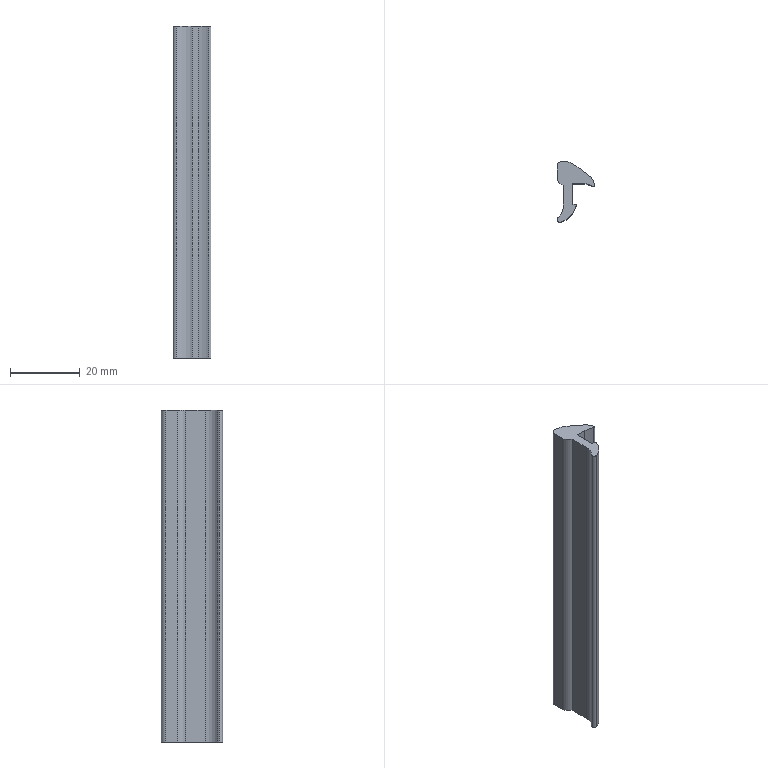Part | SolidWorks | features MoveFace 2, BaseBody 1 | 1 solid | 20 faces | box 10.8 x 17.5 x 95 mm | volume 7486 mm3 | cylinder 11 | plane 9 | commonest cylinder face diameters 1.6 x2 14 x2 0.4 x1 0.6 x1 0.8 x1 2.6 x1
STEP:
#1=CARTESIAN_POINT('',(-3.236,-11.055,115.));
#2=VERTEX_POINT('',#1);
#3=CARTESIAN_POINT('',(-4.3,-10.3,115.));
#4=VERTEX_POINT('',#3);
#5=CARTESIAN_POINT('',(-3.5,-10.3,115.));
#6=DIRECTION('',(0.,0.,-1.));
#7=DIRECTION('',(1.,0.,0.));
#8=AXIS2_PLACEMENT_3D('',#5,#6,#7);
#9=CIRCLE('',#8,0.8);
#10=EDGE_CURVE('',#2,#4,#9,.T.);
#11=ORIENTED_EDGE('',*,*,#10,.T.);
#12=CARTESIAN_POINT('',(-4.3,-10.3,20.));
#13=VERTEX_POINT('',#12);
#14=CARTESIAN_POINT('',(-4.3,-10.3,-100.));
#15=DIRECTION('',(0.,0.,-1.));
#16=VECTOR('',#15,1000.);
#17=LINE('',#14,#16);
#18=EDGE_CURVE('',#4,#13,#17,.T.);
#19=ORIENTED_EDGE('',*,*,#18,.T.);
#20=CARTESIAN_POINT('',(-3.236,-11.055,20.));
#21=VERTEX_POINT('',#20);
#22=CARTESIAN_POINT('',(-3.5,-10.3,20.));
#23=DIRECTION('',(0.,0.,1.));
#24=DIRECTION('',(1.,0.,0.));
#25=AXIS2_PLACEMENT_3D('',#22,#23,#24);
#26=CIRCLE('',#25,0.8);
#27=EDGE_CURVE('',#13,#21,#26,.T.);
#28=ORIENTED_EDGE('',*,*,#27,.T.);
#29=CARTESIAN_POINT('',(-3.236,-11.055,-100.));
#30=DIRECTION('',(0.,0.,-1.));
#31=VECTOR('',#30,1000.);
#32=LINE('',#29,#31);
#33=EDGE_CURVE('',#2,#21,#32,.T.);
#34=ORIENTED_EDGE('',*,*,#33,.F.);
#35=EDGE_LOOP('',(#11,#19,#28,#34));
#36=FACE_OUTER_BOUND('',#35,.T.);
#37=CARTESIAN_POINT('',(-3.5,-10.3,-100.));
#38=DIRECTION('',(0.,0.,-1.));
#39=DIRECTION('',(-1.,0.,0.));
#40=AXIS2_PLACEMENT_3D('',#37,#38,#39);
#41=CYLINDRICAL_SURFACE('',#40,0.8);
#42=ADVANCED_FACE('',(#36),#41,.T.);
#43=CARTESIAN_POINT('',(1.184,-6.397,20.));
#44=VERTEX_POINT('',#43);
#45=CARTESIAN_POINT('',(-5.702,-4.29,20.));
#46=DIRECTION('',(0.,0.,1.));
#47=DIRECTION('',(1.,0.,0.));
#48=AXIS2_PLACEMENT_3D('',#45,#46,#47);
#49=CIRCLE('',#48,7.201);
#50=EDGE_CURVE('',#21,#44,#49,.T.);
#51=ORIENTED_EDGE('',*,*,#50,.T.);
#52=CARTESIAN_POINT('',(1.184,-6.397,115.));
#53=VERTEX_POINT('',#52);
#54=CARTESIAN_POINT('',(1.184,-6.397,-100.));
#55=DIRECTION('',(0.,0.,1.));
#56=VECTOR('',#55,1000.);
#57=LINE('',#54,#56);
#58=EDGE_CURVE('',#44,#53,#57,.T.);
#59=ORIENTED_EDGE('',*,*,#58,.T.);
#60=CARTESIAN_POINT('',(-5.702,-4.29,115.));
#61=DIRECTION('',(0.,0.,-1.));
#62=DIRECTION('',(1.,0.,0.));
#63=AXIS2_PLACEMENT_3D('',#60,#61,#62);
#64=CIRCLE('',#63,7.201);
#65=EDGE_CURVE('',#53,#2,#64,.T.);
#66=ORIENTED_EDGE('',*,*,#65,.T.);
#67=ORIENTED_EDGE('',*,*,#33,.T.);
#68=EDGE_LOOP('',(#51,#59,#66,#67));
#69=FACE_OUTER_BOUND('',#68,.T.);
#70=CARTESIAN_POINT('',(-5.702,-4.29,-100.));
#71=DIRECTION('',(0.,0.,-1.));
#72=DIRECTION('',(-1.,0.,0.));
#73=AXIS2_PLACEMENT_3D('',#70,#71,#72);
#74=CYLINDRICAL_SURFACE('',#73,7.201);
#75=ADVANCED_FACE('',(#69),#74,.T.);
#76=CARTESIAN_POINT('',(0.9,-6.,20.));
#77=VERTEX_POINT('',#76);
#78=CARTESIAN_POINT('',(0.9,-6.3,20.));
#79=DIRECTION('',(0.,0.,1.));
#80=DIRECTION('',(1.,0.,0.));
#81=AXIS2_PLACEMENT_3D('',#78,#79,#80);
#82=CIRCLE('',#81,0.3);
#83=EDGE_CURVE('',#44,#77,#82,.T.);
#84=ORIENTED_EDGE('',*,*,#83,.T.);
#85=CARTESIAN_POINT('',(0.9,-6.,115.));
#86=VERTEX_POINT('',#85);
#87=CARTESIAN_POINT('',(0.9,-6.,-100.));
#88=DIRECTION('',(0.,0.,1.));
#89=VECTOR('',#88,1000.);
#90=LINE('',#87,#89);
#91=EDGE_CURVE('',#77,#86,#90,.T.);
#92=ORIENTED_EDGE('',*,*,#91,.T.);
#93=CARTESIAN_POINT('',(0.9,-6.3,115.));
#94=DIRECTION('',(0.,0.,-1.));
#95=DIRECTION('',(1.,0.,0.));
#96=AXIS2_PLACEMENT_3D('',#93,#94,#95);
#97=CIRCLE('',#96,0.3);
#98=EDGE_CURVE('',#86,#53,#97,.T.);
#99=ORIENTED_EDGE('',*,*,#98,.T.);
#100=ORIENTED_EDGE('',*,*,#58,.F.);
#101=EDGE_LOOP('',(#84,#92,#99,#100));
#102=FACE_OUTER_BOUND('',#101,.T.);
#103=CARTESIAN_POINT('',(0.9,-6.3,-100.));
#104=DIRECTION('',(0.,0.,-1.));
#105=DIRECTION('',(-1.,0.,0.));
#106=AXIS2_PLACEMENT_3D('',#103,#104,#105);
#107=CYLINDRICAL_SURFACE('',#106,0.3);
#108=ADVANCED_FACE('',(#102),#107,.T.);
#109=CARTESIAN_POINT('',(-2.5,-0.5,20.));
#110=VERTEX_POINT('',#109);
#111=CARTESIAN_POINT('',(-2.5,-6.153,20.));
#112=VERTEX_POINT('',#111);
#113=CARTESIAN_POINT('',(-2.5,-6.397,20.));
#114=DIRECTION('',(0.,-1.,0.));
#115=VECTOR('',#114,1000.);
#116=LINE('',#113,#115);
#117=EDGE_CURVE('',#110,#112,#116,.T.);
#118=ORIENTED_EDGE('',*,*,#117,.F.);
#119=CARTESIAN_POINT('',(-4.2,1.695,20.));
#120=VERTEX_POINT('',#119);
#121=CARTESIAN_POINT('',(-1.701,1.875,20.));
#122=DIRECTION('',(0.,0.,1.));
#123=DIRECTION('',(1.,0.,0.));
#124=AXIS2_PLACEMENT_3D('',#121,#122,#123);
#125=CIRCLE('',#124,2.506);
#126=EDGE_CURVE('',#120,#110,#125,.T.);
#127=ORIENTED_EDGE('',*,*,#126,.F.);
#128=CARTESIAN_POINT('',(-4.2,5.1,20.));
#129=VERTEX_POINT('',#128);
#130=CARTESIAN_POINT('',(-4.2,-6.397,20.));
#131=DIRECTION('',(0.,-1.,0.));
#132=VECTOR('',#131,1000.);
#133=LINE('',#130,#132);
#134=EDGE_CURVE('',#129,#120,#133,.T.);
#135=ORIENTED_EDGE('',*,*,#134,.F.);
#136=CARTESIAN_POINT('',(-2.892,6.4,20.));
#137=VERTEX_POINT('',#136);
#138=CARTESIAN_POINT('',(-2.9,5.1,20.));
#139=DIRECTION('',(0.,0.,1.));
#140=DIRECTION('',(1.,0.,0.));
#141=AXIS2_PLACEMENT_3D('',#138,#139,#140);
#142=CIRCLE('',#141,1.3);
#143=EDGE_CURVE('',#137,#129,#142,.T.);
#144=ORIENTED_EDGE('',*,*,#143,.F.);
#145=CARTESIAN_POINT('',(0.5,5.5,20.));
#146=VERTEX_POINT('',#145);
#147=CARTESIAN_POINT('',(-2.934,-0.5999,20.));
#148=DIRECTION('',(0.,0.,1.));
#149=DIRECTION('',(1.,0.,0.));
#150=AXIS2_PLACEMENT_3D('',#147,#148,#149);
#151=CIRCLE('',#150,7.);
#152=EDGE_CURVE('',#146,#137,#151,.T.);
#153=ORIENTED_EDGE('',*,*,#152,.F.);
#154=CARTESIAN_POINT('',(5.5,1.7,20.));
#155=VERTEX_POINT('',#154);
#156=CARTESIAN_POINT('',(1.595,4.668,20.));
#157=DIRECTION('',(-0.7962,0.6051,0.));
#158=VECTOR('',#157,1000.);
#159=LINE('',#156,#158);
#160=EDGE_CURVE('',#155,#146,#159,.T.);
#161=ORIENTED_EDGE('',*,*,#160,.F.);
#162=CARTESIAN_POINT('',(6.458,-0.2215,20.));
#163=VERTEX_POINT('',#162);
#164=CARTESIAN_POINT('',(6.282,0.1323,20.));
#165=DIRECTION('',(-0.4462,0.8949,0.));
#166=VECTOR('',#165,1000.);
#167=LINE('',#164,#166);
#168=EDGE_CURVE('',#163,#155,#167,.T.);
#169=ORIENTED_EDGE('',*,*,#168,.F.);
#170=CARTESIAN_POINT('',(5.895,-0.7433,20.));
#171=VERTEX_POINT('',#170);
#172=CARTESIAN_POINT('',(6.1,-0.4,20.));
#173=DIRECTION('',(0.,0.,1.));
#174=DIRECTION('',(1.,0.,0.));
#175=AXIS2_PLACEMENT_3D('',#172,#173,#174);
#176=CIRCLE('',#175,0.4);
#177=EDGE_CURVE('',#171,#163,#176,.T.);
#178=ORIENTED_EDGE('',*,*,#177,.F.);
#179=CARTESIAN_POINT('',(3.,0.,20.));
#180=VERTEX_POINT('',#179);
#181=CARTESIAN_POINT('',(2.746,-6.995,20.));
#182=DIRECTION('',(0.,0.,-1.));
#183=DIRECTION('',(1.,0.,0.));
#184=AXIS2_PLACEMENT_3D('',#181,#182,#183);
#185=CIRCLE('',#184,7.);
#186=EDGE_CURVE('',#180,#171,#185,.T.);
#187=ORIENTED_EDGE('',*,*,#186,.F.);
#188=CARTESIAN_POINT('',(0.,0.,20.));
#189=VERTEX_POINT('',#188);
#190=CARTESIAN_POINT('',(-6.814,0.,20.));
#191=DIRECTION('',(1.,0.,0.));
#192=VECTOR('',#191,1000.);
#193=LINE('',#190,#192);
#194=EDGE_CURVE('',#189,#180,#193,.T.);
#195=ORIENTED_EDGE('',*,*,#194,.F.);
#196=CARTESIAN_POINT('',(0.,-5.8,20.));
#197=VERTEX_POINT('',#196);
#198=CARTESIAN_POINT('',(0.,-6.397,20.));
#199=DIRECTION('',(0.,1.,0.));
#200=VECTOR('',#199,1000.);
#201=LINE('',#198,#200);
#202=EDGE_CURVE('',#197,#189,#201,.T.);
#203=ORIENTED_EDGE('',*,*,#202,.F.);
#204=CARTESIAN_POINT('',(0.2,-6.,20.));
#205=VERTEX_POINT('',#204);
#206=CARTESIAN_POINT('',(0.2,-5.8,20.));
#207=DIRECTION('',(0.,0.,1.));
#208=DIRECTION('',(1.,0.,0.));
#209=AXIS2_PLACEMENT_3D('',#206,#207,#208);
#210=CIRCLE('',#209,0.2);
#211=EDGE_CURVE('',#197,#205,#210,.T.);
#212=ORIENTED_EDGE('',*,*,#211,.T.);
#213=CARTESIAN_POINT('',(-6.814,-6.,20.));
#214=DIRECTION('',(-1.,0.,0.));
#215=VECTOR('',#214,1000.);
#216=LINE('',#213,#215);
#217=EDGE_CURVE('',#77,#205,#216,.T.);
#218=ORIENTED_EDGE('',*,*,#217,.F.);
#219=ORIENTED_EDGE('',*,*,#83,.F.);
#220=ORIENTED_EDGE('',*,*,#50,.F.);
#221=ORIENTED_EDGE('',*,*,#27,.F.);
#222=CARTESIAN_POINT('',(-3.998,-9.674,20.));
#223=VERTEX_POINT('',#222);
#224=CARTESIAN_POINT('',(-3.5,-10.3,20.));
#225=DIRECTION('',(0.,0.,1.));
#226=DIRECTION('',(1.,0.,0.));
#227=AXIS2_PLACEMENT_3D('',#224,#225,#226);
#228=CIRCLE('',#227,0.8);
#229=EDGE_CURVE('',#223,#13,#228,.T.);
#230=ORIENTED_EDGE('',*,*,#229,.F.);
#231=CARTESIAN_POINT('',(-6.814,-6.397,20.));
#232=DIRECTION('',(0.,0.,-1.));
#233=DIRECTION('',(1.,0.,0.));
#234=AXIS2_PLACEMENT_3D('',#231,#232,#233);
#235=CIRCLE('',#234,4.321);
#236=EDGE_CURVE('',#112,#223,#235,.T.);
#237=ORIENTED_EDGE('',*,*,#236,.F.);
#238=EDGE_LOOP('',(#118,#127,#135,#144,#153,#161,#169,#178,#187,#195,#203,#212,#218,#219,#220,#221,#230,#237));
#239=FACE_OUTER_BOUND('',#238,.T.);
#240=CARTESIAN_POINT('',(-6.814,-6.397,20.));
#241=DIRECTION('',(0.,0.,1.));
#242=DIRECTION('',(1.,0.,0.));
#243=AXIS2_PLACEMENT_3D('',#240,#241,#242);
#244=PLANE('',#243);
#245=ADVANCED_FACE('',(#239),#244,.F.);
#246=ORIENTED_EDGE('',*,*,#18,.F.);
#247=CARTESIAN_POINT('',(-3.998,-9.674,115.));
#248=VERTEX_POINT('',#247);
#249=CARTESIAN_POINT('',(-3.5,-10.3,115.));
#250=DIRECTION('',(0.,0.,-1.));
#251=DIRECTION('',(1.,0.,0.));
#252=AXIS2_PLACEMENT_3D('',#249,#250,#251);
#253=CIRCLE('',#252,0.8);
#254=EDGE_CURVE('',#4,#248,#253,.T.);
#255=ORIENTED_EDGE('',*,*,#254,.T.);
#256=CARTESIAN_POINT('',(-3.998,-9.674,-100.));
#257=DIRECTION('',(0.,0.,-1.));
#258=VECTOR('',#257,1000.);
#259=LINE('',#256,#258);
#260=EDGE_CURVE('',#248,#223,#259,.T.);
#261=ORIENTED_EDGE('',*,*,#260,.T.);
#262=ORIENTED_EDGE('',*,*,#229,.T.);
#263=EDGE_LOOP('',(#246,#255,#261,#262));
#264=FACE_OUTER_BOUND('',#263,.T.);
#265=CARTESIAN_POINT('',(-3.5,-10.3,-100.));
#266=DIRECTION('',(0.,0.,-1.));
#267=DIRECTION('',(-1.,0.,0.));
#268=AXIS2_PLACEMENT_3D('',#265,#266,#267);
#269=CYLINDRICAL_SURFACE('',#268,0.8);
#270=ADVANCED_FACE('',(#264),#269,.T.);
#271=CARTESIAN_POINT('',(-4.2,1.695,115.));
#272=VERTEX_POINT('',#271);
#273=CARTESIAN_POINT('',(-2.5,-0.5,115.));
#274=VERTEX_POINT('',#273);
#275=CARTESIAN_POINT('',(-1.701,1.875,115.));
#276=DIRECTION('',(0.,0.,1.));
#277=DIRECTION('',(1.,0.,0.));
#278=AXIS2_PLACEMENT_3D('',#275,#276,#277);
#279=CIRCLE('',#278,2.506);
#280=EDGE_CURVE('',#272,#274,#279,.T.);
#281=ORIENTED_EDGE('',*,*,#280,.T.);
#282=CARTESIAN_POINT('',(-2.5,-6.153,115.));
#283=VERTEX_POINT('',#282);
#284=CARTESIAN_POINT('',(-2.5,-6.397,115.));
#285=DIRECTION('',(0.,-1.,0.));
#286=VECTOR('',#285,1000.);
#287=LINE('',#284,#286);
#288=EDGE_CURVE('',#274,#283,#287,.T.);
#289=ORIENTED_EDGE('',*,*,#288,.T.);
#290=CARTESIAN_POINT('',(-6.814,-6.397,115.));
#291=DIRECTION('',(0.,0.,-1.));
#292=DIRECTION('',(1.,0.,0.));
#293=AXIS2_PLACEMENT_3D('',#290,#291,#292);
#294=CIRCLE('',#293,4.321);
#295=EDGE_CURVE('',#283,#248,#294,.T.);
#296=ORIENTED_EDGE('',*,*,#295,.T.);
#297=ORIENTED_EDGE('',*,*,#254,.F.);
#298=ORIENTED_EDGE('',*,*,#10,.F.);
#299=ORIENTED_EDGE('',*,*,#65,.F.);
#300=ORIENTED_EDGE('',*,*,#98,.F.);
#301=CARTESIAN_POINT('',(0.2,-6.,115.));
#302=VERTEX_POINT('',#301);
#303=CARTESIAN_POINT('',(-6.814,-6.,115.));
#304=DIRECTION('',(-1.,0.,0.));
#305=VECTOR('',#304,1000.);
#306=LINE('',#303,#305);
#307=EDGE_CURVE('',#86,#302,#306,.T.);
#308=ORIENTED_EDGE('',*,*,#307,.T.);
#309=CARTESIAN_POINT('',(0.,-5.8,115.));
#310=VERTEX_POINT('',#309);
#311=CARTESIAN_POINT('',(0.2,-5.8,115.));
#312=DIRECTION('',(0.,0.,-1.));
#313=DIRECTION('',(1.,0.,0.));
#314=AXIS2_PLACEMENT_3D('',#311,#312,#313);
#315=CIRCLE('',#314,0.2);
#316=EDGE_CURVE('',#302,#310,#315,.T.);
#317=ORIENTED_EDGE('',*,*,#316,.T.);
#318=CARTESIAN_POINT('',(0.,0.,115.));
#319=VERTEX_POINT('',#318);
#320=CARTESIAN_POINT('',(0.,-6.397,115.));
#321=DIRECTION('',(0.,1.,0.));
#322=VECTOR('',#321,1000.);
#323=LINE('',#320,#322);
#324=EDGE_CURVE('',#310,#319,#323,.T.);
#325=ORIENTED_EDGE('',*,*,#324,.T.);
#326=CARTESIAN_POINT('',(3.,0.,115.));
#327=VERTEX_POINT('',#326);
#328=CARTESIAN_POINT('',(-6.814,0.,115.));
#329=DIRECTION('',(1.,0.,0.));
#330=VECTOR('',#329,1000.);
#331=LINE('',#328,#330);
#332=EDGE_CURVE('',#319,#327,#331,.T.);
#333=ORIENTED_EDGE('',*,*,#332,.T.);
#334=CARTESIAN_POINT('',(5.895,-0.7433,115.));
#335=VERTEX_POINT('',#334);
#336=CARTESIAN_POINT('',(2.746,-6.995,115.));
#337=DIRECTION('',(0.,0.,-1.));
#338=DIRECTION('',(1.,0.,0.));
#339=AXIS2_PLACEMENT_3D('',#336,#337,#338);
#340=CIRCLE('',#339,7.);
#341=EDGE_CURVE('',#327,#335,#340,.T.);
#342=ORIENTED_EDGE('',*,*,#341,.T.);
#343=CARTESIAN_POINT('',(6.458,-0.2215,115.));
#344=VERTEX_POINT('',#343);
#345=CARTESIAN_POINT('',(6.1,-0.4,115.));
#346=DIRECTION('',(0.,0.,-1.));
#347=DIRECTION('',(1.,0.,0.));
#348=AXIS2_PLACEMENT_3D('',#345,#346,#347);
#349=CIRCLE('',#348,0.4);
#350=EDGE_CURVE('',#344,#335,#349,.T.);
#351=ORIENTED_EDGE('',*,*,#350,.F.);
#352=CARTESIAN_POINT('',(5.5,1.7,115.));
#353=VERTEX_POINT('',#352);
#354=CARTESIAN_POINT('',(6.282,0.1323,115.));
#355=DIRECTION('',(-0.4462,0.8949,0.));
#356=VECTOR('',#355,1000.);
#357=LINE('',#354,#356);
#358=EDGE_CURVE('',#344,#353,#357,.T.);
#359=ORIENTED_EDGE('',*,*,#358,.T.);
#360=CARTESIAN_POINT('',(0.5,5.5,115.));
#361=VERTEX_POINT('',#360);
#362=CARTESIAN_POINT('',(1.595,4.668,115.));
#363=DIRECTION('',(-0.7962,0.6051,0.));
#364=VECTOR('',#363,1000.);
#365=LINE('',#362,#364);
#366=EDGE_CURVE('',#353,#361,#365,.T.);
#367=ORIENTED_EDGE('',*,*,#366,.T.);
#368=CARTESIAN_POINT('',(-2.892,6.4,115.));
#369=VERTEX_POINT('',#368);
#370=CARTESIAN_POINT('',(-2.934,-0.5999,115.));
#371=DIRECTION('',(0.,0.,1.));
#372=DIRECTION('',(1.,0.,0.));
#373=AXIS2_PLACEMENT_3D('',#370,#371,#372);
#374=CIRCLE('',#373,7.);
#375=EDGE_CURVE('',#361,#369,#374,.T.);
#376=ORIENTED_EDGE('',*,*,#375,.T.);
#377=CARTESIAN_POINT('',(-4.2,5.1,115.));
#378=VERTEX_POINT('',#377);
#379=CARTESIAN_POINT('',(-2.9,5.1,115.));
#380=DIRECTION('',(0.,0.,1.));
#381=DIRECTION('',(1.,0.,0.));
#382=AXIS2_PLACEMENT_3D('',#379,#380,#381);
#383=CIRCLE('',#382,1.3);
#384=EDGE_CURVE('',#369,#378,#383,.T.);
#385=ORIENTED_EDGE('',*,*,#384,.T.);
#386=CARTESIAN_POINT('',(-4.2,-6.397,115.));
#387=DIRECTION('',(0.,-1.,0.));
#388=VECTOR('',#387,1000.);
#389=LINE('',#386,#388);
#390=EDGE_CURVE('',#378,#272,#389,.T.);
#391=ORIENTED_EDGE('',*,*,#390,.T.);
#392=EDGE_LOOP('',(#281,#289,#296,#297,#298,#299,#300,#308,#317,#325,#333,#342,#351,#359,#367,#376,#385,#391));
#393=FACE_OUTER_BOUND('',#392,.T.);
#394=CARTESIAN_POINT('',(-6.814,-6.397,115.));
#395=DIRECTION('',(0.,0.,1.));
#396=DIRECTION('',(1.,0.,0.));
#397=AXIS2_PLACEMENT_3D('',#394,#395,#396);
#398=PLANE('',#397);
#399=ADVANCED_FACE('',(#393),#398,.T.);
#400=ORIENTED_EDGE('',*,*,#217,.T.);
#401=CARTESIAN_POINT('',(0.2,-6.,-100.));
#402=DIRECTION('',(0.,0.,1.));
#403=VECTOR('',#402,1000.);
#404=LINE('',#401,#403);
#405=EDGE_CURVE('',#205,#302,#404,.T.);
#406=ORIENTED_EDGE('',*,*,#405,.T.);
#407=ORIENTED_EDGE('',*,*,#307,.F.);
#408=ORIENTED_EDGE('',*,*,#91,.F.);
#409=EDGE_LOOP('',(#400,#406,#407,#408));
#410=FACE_OUTER_BOUND('',#409,.T.);
#411=CARTESIAN_POINT('',(0.9,-6.,-100.));
#412=DIRECTION('',(0.,1.,0.));
#413=DIRECTION('',(0.,0.,1.));
#414=AXIS2_PLACEMENT_3D('',#411,#412,#413);
#415=PLANE('',#414);
#416=ADVANCED_FACE('',(#410),#415,.T.);
#417=CARTESIAN_POINT('',(-2.5,-6.153,-100.));
#418=DIRECTION('',(0.,0.,1.));
#419=VECTOR('',#418,1000.);
#420=LINE('',#417,#419);
#421=EDGE_CURVE('',#112,#283,#420,.T.);
#422=ORIENTED_EDGE('',*,*,#421,.F.);
#423=ORIENTED_EDGE('',*,*,#236,.T.);
#424=ORIENTED_EDGE('',*,*,#260,.F.);
#425=ORIENTED_EDGE('',*,*,#295,.F.);
#426=EDGE_LOOP('',(#422,#423,#424,#425));
#427=FACE_OUTER_BOUND('',#426,.T.);
#428=CARTESIAN_POINT('',(-6.814,-6.397,-100.));
#429=DIRECTION('',(0.,0.,-1.));
#430=DIRECTION('',(-1.,0.,0.));
#431=AXIS2_PLACEMENT_3D('',#428,#429,#430);
#432=CYLINDRICAL_SURFACE('',#431,4.321);
#433=ADVANCED_FACE('',(#427),#432,.F.);
#434=ORIENTED_EDGE('',*,*,#117,.T.);
#435=ORIENTED_EDGE('',*,*,#421,.T.);
#436=ORIENTED_EDGE('',*,*,#288,.F.);
#437=CARTESIAN_POINT('',(-2.5,-0.5,-100.));
#438=DIRECTION('',(0.,0.,-1.));
#439=VECTOR('',#438,1000.);
#440=LINE('',#437,#439);
#441=EDGE_CURVE('',#274,#110,#440,.T.);
#442=ORIENTED_EDGE('',*,*,#441,.T.);
#443=EDGE_LOOP('',(#434,#435,#436,#442));
#444=FACE_OUTER_BOUND('',#443,.T.);
#445=CARTESIAN_POINT('',(-2.5,-0.5,-100.));
#446=DIRECTION('',(-1.,0.,0.));
#447=DIRECTION('',(0.,0.,1.));
#448=AXIS2_PLACEMENT_3D('',#445,#446,#447);
#449=PLANE('',#448);
#450=ADVANCED_FACE('',(#444),#449,.T.);
#451=ORIENTED_EDGE('',*,*,#126,.T.);
#452=ORIENTED_EDGE('',*,*,#441,.F.);
#453=ORIENTED_EDGE('',*,*,#280,.F.);
#454=CARTESIAN_POINT('',(-4.2,1.695,-100.));
#455=DIRECTION('',(0.,0.,-1.));
#456=VECTOR('',#455,1000.);
#457=LINE('',#454,#456);
#458=EDGE_CURVE('',#272,#120,#457,.T.);
#459=ORIENTED_EDGE('',*,*,#458,.T.);
#460=EDGE_LOOP('',(#451,#452,#453,#459));
#461=FACE_OUTER_BOUND('',#460,.T.);
#462=CARTESIAN_POINT('',(-1.701,1.875,-100.));
#463=DIRECTION('',(0.,0.,-1.));
#464=DIRECTION('',(-1.,0.,0.));
#465=AXIS2_PLACEMENT_3D('',#462,#463,#464);
#466=CYLINDRICAL_SURFACE('',#465,2.506);
#467=ADVANCED_FACE('',(#461),#466,.T.);
#468=ORIENTED_EDGE('',*,*,#134,.T.);
#469=ORIENTED_EDGE('',*,*,#458,.F.);
#470=ORIENTED_EDGE('',*,*,#390,.F.);
#471=CARTESIAN_POINT('',(-4.2,5.1,-100.));
#472=DIRECTION('',(0.,0.,-1.));
#473=VECTOR('',#472,1000.);
#474=LINE('',#471,#473);
#475=EDGE_CURVE('',#378,#129,#474,.T.);
#476=ORIENTED_EDGE('',*,*,#475,.T.);
#477=EDGE_LOOP('',(#468,#469,#470,#476));
#478=FACE_OUTER_BOUND('',#477,.T.);
#479=CARTESIAN_POINT('',(-4.2,5.1,-100.));
#480=DIRECTION('',(-1.,0.,0.));
#481=DIRECTION('',(0.,0.,1.));
#482=AXIS2_PLACEMENT_3D('',#479,#480,#481);
#483=PLANE('',#482);
#484=ADVANCED_FACE('',(#478),#483,.T.);
#485=ORIENTED_EDGE('',*,*,#143,.T.);
#486=ORIENTED_EDGE('',*,*,#475,.F.);
#487=ORIENTED_EDGE('',*,*,#384,.F.);
#488=CARTESIAN_POINT('',(-2.892,6.4,-100.));
#489=DIRECTION('',(0.,0.,-1.));
#490=VECTOR('',#489,1000.);
#491=LINE('',#488,#490);
#492=EDGE_CURVE('',#369,#137,#491,.T.);
#493=ORIENTED_EDGE('',*,*,#492,.T.);
#494=EDGE_LOOP('',(#485,#486,#487,#493));
#495=FACE_OUTER_BOUND('',#494,.T.);
#496=CARTESIAN_POINT('',(-2.9,5.1,-100.));
#497=DIRECTION('',(0.,0.,-1.));
#498=DIRECTION('',(-1.,0.,0.));
#499=AXIS2_PLACEMENT_3D('',#496,#497,#498);
#500=CYLINDRICAL_SURFACE('',#499,1.3);
#501=ADVANCED_FACE('',(#495),#500,.T.);
#502=ORIENTED_EDGE('',*,*,#152,.T.);
#503=ORIENTED_EDGE('',*,*,#492,.F.);
#504=ORIENTED_EDGE('',*,*,#375,.F.);
#505=CARTESIAN_POINT('',(0.5,5.5,-100.));
#506=DIRECTION('',(0.,0.,-1.));
#507=VECTOR('',#506,1000.);
#508=LINE('',#505,#507);
#509=EDGE_CURVE('',#361,#146,#508,.T.);
#510=ORIENTED_EDGE('',*,*,#509,.T.);
#511=EDGE_LOOP('',(#502,#503,#504,#510));
#512=FACE_OUTER_BOUND('',#511,.T.);
#513=CARTESIAN_POINT('',(-2.934,-0.5999,-100.));
#514=DIRECTION('',(0.,0.,-1.));
#515=DIRECTION('',(-1.,0.,0.));
#516=AXIS2_PLACEMENT_3D('',#513,#514,#515);
#517=CYLINDRICAL_SURFACE('',#516,7.);
#518=ADVANCED_FACE('',(#512),#517,.T.);
#519=ORIENTED_EDGE('',*,*,#160,.T.);
#520=ORIENTED_EDGE('',*,*,#509,.F.);
#521=ORIENTED_EDGE('',*,*,#366,.F.);
#522=CARTESIAN_POINT('',(5.5,1.7,-100.));
#523=DIRECTION('',(0.,0.,-1.));
#524=VECTOR('',#523,1000.);
#525=LINE('',#522,#524);
#526=EDGE_CURVE('',#353,#155,#525,.T.);
#527=ORIENTED_EDGE('',*,*,#526,.T.);
#528=EDGE_LOOP('',(#519,#520,#521,#527));
#529=FACE_OUTER_BOUND('',#528,.T.);
#530=CARTESIAN_POINT('',(5.5,1.7,-100.));
#531=DIRECTION('',(0.6051,0.7962,0.));
#532=DIRECTION('',(-0.7962,0.6051,0.));
#533=AXIS2_PLACEMENT_3D('',#530,#531,#532);
#534=PLANE('',#533);
#535=ADVANCED_FACE('',(#529),#534,.T.);
#536=ORIENTED_EDGE('',*,*,#168,.T.);
#537=ORIENTED_EDGE('',*,*,#526,.F.);
#538=ORIENTED_EDGE('',*,*,#358,.F.);
#539=CARTESIAN_POINT('',(6.458,-0.2215,-100.));
#540=DIRECTION('',(0.,0.,-1.));
#541=VECTOR('',#540,1000.);
#542=LINE('',#539,#541);
#543=EDGE_CURVE('',#344,#163,#542,.T.);
#544=ORIENTED_EDGE('',*,*,#543,.T.);
#545=EDGE_LOOP('',(#536,#537,#538,#544));
#546=FACE_OUTER_BOUND('',#545,.T.);
#547=CARTESIAN_POINT('',(6.458,-0.2215,-100.));
#548=DIRECTION('',(0.8949,0.4462,0.));
#549=DIRECTION('',(-0.4462,0.8949,0.));
#550=AXIS2_PLACEMENT_3D('',#547,#548,#549);
#551=PLANE('',#550);
#552=ADVANCED_FACE('',(#546),#551,.T.);
#553=CARTESIAN_POINT('',(3.,0.,-100.));
#554=DIRECTION('',(0.,0.,1.));
#555=VECTOR('',#554,1000.);
#556=LINE('',#553,#555);
#557=EDGE_CURVE('',#180,#327,#556,.T.);
#558=ORIENTED_EDGE('',*,*,#557,.F.);
#559=ORIENTED_EDGE('',*,*,#186,.T.);
#560=CARTESIAN_POINT('',(5.895,-0.7433,-100.));
#561=DIRECTION('',(0.,0.,-1.));
#562=VECTOR('',#561,1000.);
#563=LINE('',#560,#562);
#564=EDGE_CURVE('',#335,#171,#563,.T.);
#565=ORIENTED_EDGE('',*,*,#564,.F.);
#566=ORIENTED_EDGE('',*,*,#341,.F.);
#567=EDGE_LOOP('',(#558,#559,#565,#566));
#568=FACE_OUTER_BOUND('',#567,.T.);
#569=CARTESIAN_POINT('',(2.746,-6.995,-100.));
#570=DIRECTION('',(0.,0.,-1.));
#571=DIRECTION('',(-1.,0.,0.));
#572=AXIS2_PLACEMENT_3D('',#569,#570,#571);
#573=CYLINDRICAL_SURFACE('',#572,7.);
#574=ADVANCED_FACE('',(#568),#573,.F.);
#575=ORIENTED_EDGE('',*,*,#194,.T.);
#576=ORIENTED_EDGE('',*,*,#557,.T.);
#577=ORIENTED_EDGE('',*,*,#332,.F.);
#578=CARTESIAN_POINT('',(0.,0.,-100.));
#579=DIRECTION('',(0.,0.,-1.));
#580=VECTOR('',#579,1000.);
#581=LINE('',#578,#580);
#582=EDGE_CURVE('',#319,#189,#581,.T.);
#583=ORIENTED_EDGE('',*,*,#582,.T.);
#584=EDGE_LOOP('',(#575,#576,#577,#583));
#585=FACE_OUTER_BOUND('',#584,.T.);
#586=CARTESIAN_POINT('',(0.,0.,-100.));
#587=DIRECTION('',(0.,-1.,0.));
#588=DIRECTION('',(0.,0.,-1.));
#589=AXIS2_PLACEMENT_3D('',#586,#587,#588);
#590=PLANE('',#589);
#591=ADVANCED_FACE('',(#585),#590,.T.);
#592=ORIENTED_EDGE('',*,*,#202,.T.);
#593=ORIENTED_EDGE('',*,*,#582,.F.);
#594=ORIENTED_EDGE('',*,*,#324,.F.);
#595=CARTESIAN_POINT('',(0.,-5.8,-100.));
#596=DIRECTION('',(0.,0.,-1.));
#597=VECTOR('',#596,1000.);
#598=LINE('',#595,#597);
#599=EDGE_CURVE('',#310,#197,#598,.T.);
#600=ORIENTED_EDGE('',*,*,#599,.T.);
#601=EDGE_LOOP('',(#592,#593,#594,#600));
#602=FACE_OUTER_BOUND('',#601,.T.);
#603=CARTESIAN_POINT('',(0.,-5.8,-100.));
#604=DIRECTION('',(1.,0.,0.));
#605=DIRECTION('',(0.,0.,-1.));
#606=AXIS2_PLACEMENT_3D('',#603,#604,#605);
#607=PLANE('',#606);
#608=ADVANCED_FACE('',(#602),#607,.T.);
#609=ORIENTED_EDGE('',*,*,#405,.F.);
#610=ORIENTED_EDGE('',*,*,#211,.F.);
#611=ORIENTED_EDGE('',*,*,#599,.F.);
#612=ORIENTED_EDGE('',*,*,#316,.F.);
#613=EDGE_LOOP('',(#609,#610,#611,#612));
#614=FACE_OUTER_BOUND('',#613,.T.);
#615=CARTESIAN_POINT('',(0.2,-5.8,-100.));
#616=DIRECTION('',(0.,0.,-1.));
#617=DIRECTION('',(-1.,0.,0.));
#618=AXIS2_PLACEMENT_3D('',#615,#616,#617);
#619=CYLINDRICAL_SURFACE('',#618,0.2);
#620=ADVANCED_FACE('',(#614),#619,.F.);
#621=ORIENTED_EDGE('',*,*,#177,.T.);
#622=ORIENTED_EDGE('',*,*,#543,.F.);
#623=ORIENTED_EDGE('',*,*,#350,.T.);
#624=ORIENTED_EDGE('',*,*,#564,.T.);
#625=EDGE_LOOP('',(#621,#622,#623,#624));
#626=FACE_OUTER_BOUND('',#625,.T.);
#627=CARTESIAN_POINT('',(6.1,-0.4,-100.));
#628=DIRECTION('',(0.,0.,-1.));
#629=DIRECTION('',(-1.,0.,0.));
#630=AXIS2_PLACEMENT_3D('',#627,#628,#629);
#631=CYLINDRICAL_SURFACE('',#630,0.4);
#632=ADVANCED_FACE('',(#626),#631,.T.);
#633=CLOSED_SHELL('',(#42,#75,#108,#245,#270,#399,#416,#433,#450,#467,#484,#501,#518,#535,#552,#574,#591,#608,#620,#632));
#634=MANIFOLD_SOLID_BREP('',#633);
#635=CARTESIAN_POINT('',(0.,0.,0.));
#636=DIRECTION('',(0.,0.,1.));
#637=DIRECTION('',(1.,0.,0.));
#638=AXIS2_PLACEMENT_3D('',#635,#636,#637);
#639=(LENGTH_UNIT()NAMED_UNIT(*)SI_UNIT(.MILLI.,.METRE.));
#640=UNCERTAINTY_MEASURE_WITH_UNIT(LENGTH_MEASURE(0.00001),#639,'','');
#641=(NAMED_UNIT(*)PLANE_ANGLE_UNIT()SI_UNIT($,.RADIAN.));
#642=(NAMED_UNIT(*)SI_UNIT($,.STERADIAN.)SOLID_ANGLE_UNIT());
#643=(GEOMETRIC_REPRESENTATION_CONTEXT(3)GLOBAL_UNCERTAINTY_ASSIGNED_CONTEXT((#640))GLOBAL_UNIT_ASSIGNED_CONTEXT((#639,#641,#642))REPRESENTATION_CONTEXT('',''));
#644=ADVANCED_BREP_SHAPE_REPRESENTATION('',(#634,#638),#643);